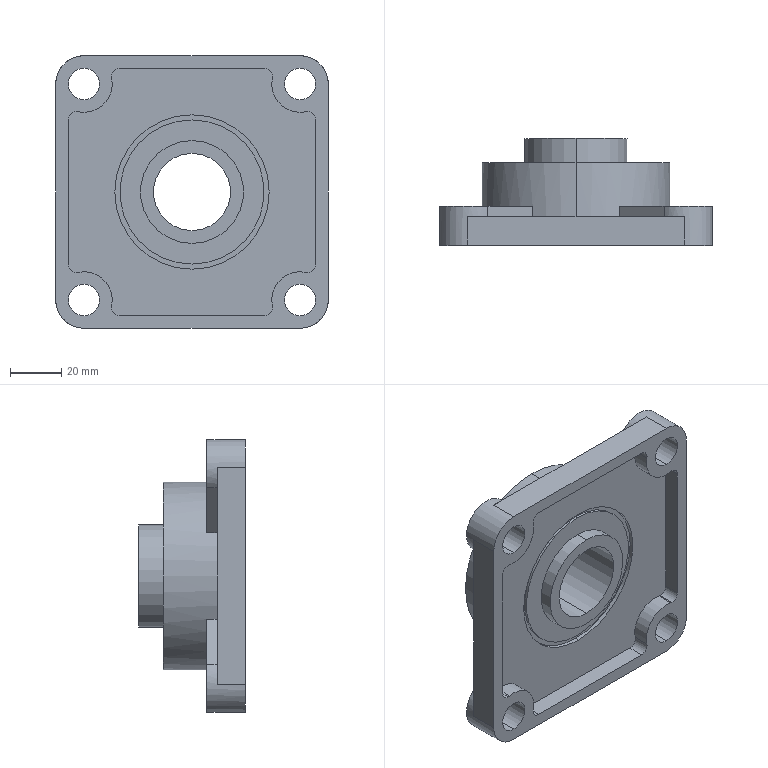Part | STEP file | Bearing housing F206 | 4 solids | 82 faces | box 106 x 41.5 x 106 mm | volume 142901 mm3 | cylinder 48 | plane 34 | commonest cylinder face diameters 22 x12 6 x10 12.2 x8 40 x4 56 x4 60 x4